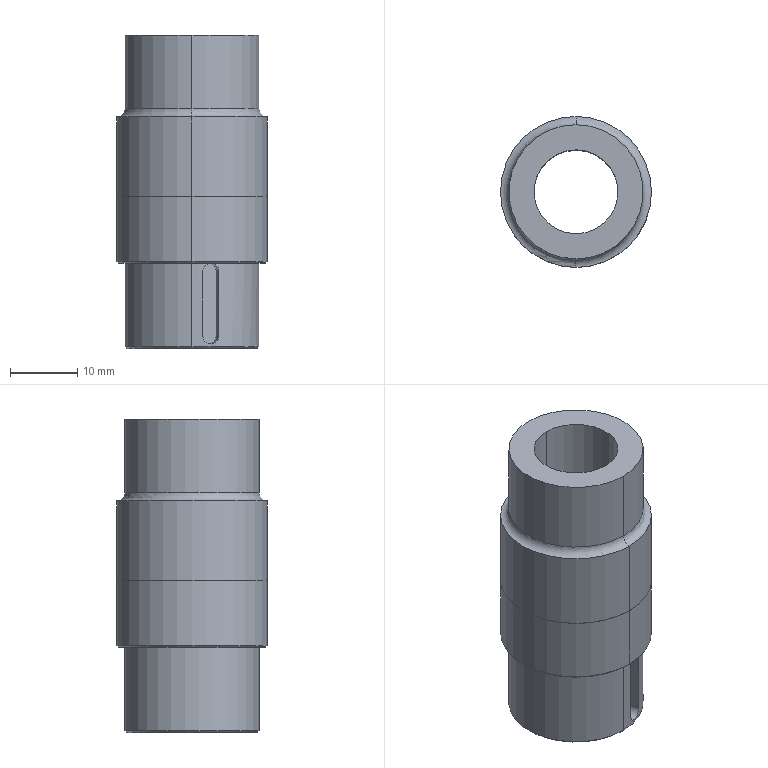Part | STEP file | 2026.6.15-Main Assembly图.sldasm-Part-96 | 1 solid | 32 faces | box 22.5 x 22.5 x 46.645 mm | volume 10487 mm3 | cylinder 16 | plane 8 | cone 6 | torus 2 | commonest cylinder face diameters 2.5 x4 20 x4 12.5 x2 14 x2 22.45 x2 22.5 x2
STEP:
#1=CARTESIAN_POINT('',(-1569.631,1414.394,3480.447));
#2=VERTEX_POINT('',#1);
#3=CARTESIAN_POINT('',(-1569.631,1414.394,3480.441));
#4=VERTEX_POINT('',#3);
#5=CARTESIAN_POINT('',(-1569.631,1414.394,3480.447));
#6=CARTESIAN_POINT('',(-1569.631,1414.394,3480.445));
#7=CARTESIAN_POINT('',(-1569.631,1414.394,3480.443));
#8=CARTESIAN_POINT('',(-1569.631,1414.394,3480.441));
#9=B_SPLINE_CURVE_WITH_KNOTS('',3,(#5,#6,#7,#8),.UNSPECIFIED.,.F.,.F.,(4,4),(0.,0.000005656),.UNSPECIFIED.);
#10=EDGE_CURVE('',#2,#4,#9,.T.);
#11=ORIENTED_EDGE('',*,*,#10,.T.);
#12=CARTESIAN_POINT('',(-1570.033,1415.758,3480.441));
#13=VERTEX_POINT('',#12);
#14=CARTESIAN_POINT('',(-1570.033,1415.758,3480.441));
#15=DIRECTION('',(-0.2829,0.9592,0.));
#16=VECTOR('',#15,1000.);
#17=LINE('',#14,#16);
#18=EDGE_CURVE('',#4,#13,#17,.T.);
#19=ORIENTED_EDGE('',*,*,#18,.T.);
#20=CARTESIAN_POINT('',(-1570.033,1415.758,3480.447));
#21=VERTEX_POINT('',#20);
#22=CARTESIAN_POINT('',(-1568.834,1416.111,3480.447));
#23=DIRECTION('',(0.2829,-0.9592,0.));
#24=DIRECTION('',(-0.9591,-0.2829,-0.004589));
#25=AXIS2_PLACEMENT_3D('',#22,#23,#24);
#26=CIRCLE('',#25,1.25);
#27=EDGE_CURVE('',#21,#13,#26,.T.);
#28=ORIENTED_EDGE('',*,*,#27,.F.);
#29=CARTESIAN_POINT('',(-1570.033,1415.758,3480.447));
#30=DIRECTION('',(-0.2829,0.9592,0.));
#31=VECTOR('',#30,1000.);
#32=LINE('',#29,#31);
#33=EDGE_CURVE('',#2,#21,#32,.T.);
#34=ORIENTED_EDGE('',*,*,#33,.F.);
#35=EDGE_LOOP('',(#11,#19,#28,#34));
#36=FACE_OUTER_BOUND('',#35,.T.);
#37=CARTESIAN_POINT('',(-1568.834,1416.111,3480.447));
#38=DIRECTION('',(-0.2829,0.9592,0.));
#39=DIRECTION('',(-0.9591,-0.2829,-0.004589));
#40=AXIS2_PLACEMENT_3D('',#37,#38,#39);
#41=CYLINDRICAL_SURFACE('',#40,1.25);
#42=ADVANCED_FACE('',(#36),#41,.F.);
#43=CARTESIAN_POINT('',(-1567.635,1416.465,3489.953));
#44=VERTEX_POINT('',#43);
#45=CARTESIAN_POINT('',(-1570.033,1415.758,3489.947));
#46=VERTEX_POINT('',#45);
#47=CARTESIAN_POINT('',(-1568.834,1416.111,3489.947));
#48=DIRECTION('',(0.2829,-0.9592,0.));
#49=DIRECTION('',(-0.9591,-0.2829,-0.004589));
#50=AXIS2_PLACEMENT_3D('',#47,#48,#49);
#51=CIRCLE('',#50,1.25);
#52=EDGE_CURVE('',#44,#46,#51,.T.);
#53=ORIENTED_EDGE('',*,*,#52,.F.);
#54=CARTESIAN_POINT('',(-1567.233,1415.102,3489.953));
#55=VERTEX_POINT('',#54);
#56=CARTESIAN_POINT('',(-1567.635,1416.465,3489.953));
#57=DIRECTION('',(0.2829,-0.9592,0.));
#58=VECTOR('',#57,1000.);
#59=LINE('',#56,#58);
#60=EDGE_CURVE('',#44,#55,#59,.T.);
#61=ORIENTED_EDGE('',*,*,#60,.T.);
#62=CARTESIAN_POINT('',(-1568.41,1414.673,3491.197));
#63=VERTEX_POINT('',#62);
#64=CARTESIAN_POINT('',(-1567.233,1415.102,3489.953));
#65=CARTESIAN_POINT('',(-1567.234,1415.101,3490.117));
#66=CARTESIAN_POINT('',(-1567.264,1415.088,3490.279));
#67=CARTESIAN_POINT('',(-1567.381,1415.038,3490.58));
#68=CARTESIAN_POINT('',(-1567.467,1415.002,3490.718));
#69=CARTESIAN_POINT('',(-1567.683,1414.917,3490.948));
#70=CARTESIAN_POINT('',(-1567.813,1414.868,3491.04));
#71=CARTESIAN_POINT('',(-1568.097,1414.769,3491.164));
#72=CARTESIAN_POINT('',(-1568.253,1414.719,3491.197));
#73=CARTESIAN_POINT('',(-1568.41,1414.673,3491.197));
#74=B_SPLINE_CURVE_WITH_KNOTS('',3,(#64,#65,#66,#67,#68,#69,#70,#71,#72,#73),.UNSPECIFIED.,.F.,.F.,(4,2,2,2,4),(0.000005656,0.0004933,0.000981,0.001469,0.001956),.UNSPECIFIED.);
#75=EDGE_CURVE('',#55,#63,#74,.T.);
#76=ORIENTED_EDGE('',*,*,#75,.T.);
#77=CARTESIAN_POINT('',(-1569.631,1414.394,3489.947));
#78=VERTEX_POINT('',#77);
#79=CARTESIAN_POINT('',(-1568.41,1414.673,3491.197));
#80=CARTESIAN_POINT('',(-1568.488,1414.65,3491.197));
#81=CARTESIAN_POINT('',(-1568.568,1414.627,3491.189));
#82=CARTESIAN_POINT('',(-1568.722,1414.586,3491.157));
#83=CARTESIAN_POINT('',(-1568.798,1414.566,3491.133));
#84=CARTESIAN_POINT('',(-1569.019,1414.513,3491.039));
#85=CARTESIAN_POINT('',(-1569.153,1414.483,3490.947));
#86=CARTESIAN_POINT('',(-1569.383,1414.437,3490.714));
#87=CARTESIAN_POINT('',(-1569.474,1414.421,3490.577));
#88=CARTESIAN_POINT('',(-1569.598,1414.4,3490.275));
#89=CARTESIAN_POINT('',(-1569.631,1414.394,3490.112));
#90=CARTESIAN_POINT('',(-1569.631,1414.394,3489.947));
#91=B_SPLINE_CURVE_WITH_KNOTS('',3,(#79,#80,#81,#82,#83,#84,#85,#86,#87,#88,#89,#90),.UNSPECIFIED.,.F.,.F.,(4,2,2,2,2,4),(0.001956,0.002201,0.002445,0.002934,0.003422,0.003911),.UNSPECIFIED.);
#92=EDGE_CURVE('',#63,#78,#91,.T.);
#93=ORIENTED_EDGE('',*,*,#92,.T.);
#94=CARTESIAN_POINT('',(-1570.033,1415.758,3489.947));
#95=DIRECTION('',(0.2829,-0.9592,0.));
#96=VECTOR('',#95,1000.);
#97=LINE('',#94,#96);
#98=EDGE_CURVE('',#46,#78,#97,.T.);
#99=ORIENTED_EDGE('',*,*,#98,.F.);
#100=EDGE_LOOP('',(#53,#61,#76,#93,#99));
#101=FACE_OUTER_BOUND('',#100,.T.);
#102=CARTESIAN_POINT('',(-1568.834,1416.111,3489.947));
#103=DIRECTION('',(0.2829,-0.9592,0.));
#104=DIRECTION('',(0.9591,0.2829,0.004589));
#105=AXIS2_PLACEMENT_3D('',#102,#103,#104);
#106=CYLINDRICAL_SURFACE('',#105,1.25);
#107=ADVANCED_FACE('',(#101),#106,.F.);
#108=CARTESIAN_POINT('',(-1571.247,1413.014,3501.197));
#109=VERTEX_POINT('',#108);
#110=CARTESIAN_POINT('',(-1571.23,1435.514,3501.197));
#111=VERTEX_POINT('',#110);
#112=CARTESIAN_POINT('',(-1571.238,1424.264,3501.197));
#113=DIRECTION('',(0.,0.,1.));
#114=DIRECTION('',(-0.0007664,-1.,0.));
#115=AXIS2_PLACEMENT_3D('',#112,#113,#114);
#116=CIRCLE('',#115,11.25);
#117=EDGE_CURVE('',#109,#111,#116,.T.);
#118=ORIENTED_EDGE('',*,*,#117,.T.);
#119=CARTESIAN_POINT('',(-1571.23,1435.514,3512.997));
#120=VERTEX_POINT('',#119);
#121=CARTESIAN_POINT('',(-1571.23,1435.514,3478.747));
#122=DIRECTION('',(0.,0.,1.));
#123=VECTOR('',#122,1000.);
#124=LINE('',#121,#123);
#125=EDGE_CURVE('',#111,#120,#124,.T.);
#126=ORIENTED_EDGE('',*,*,#125,.T.);
#127=CARTESIAN_POINT('',(-1571.247,1413.014,3512.997));
#128=VERTEX_POINT('',#127);
#129=CARTESIAN_POINT('',(-1571.238,1424.264,3512.997));
#130=DIRECTION('',(0.,0.,1.));
#131=DIRECTION('',(-0.0007664,-1.,0.));
#132=AXIS2_PLACEMENT_3D('',#129,#130,#131);
#133=CIRCLE('',#132,11.25);
#134=EDGE_CURVE('',#128,#120,#133,.T.);
#135=ORIENTED_EDGE('',*,*,#134,.F.);
#136=CARTESIAN_POINT('',(-1571.247,1413.014,3478.747));
#137=DIRECTION('',(0.,0.,1.));
#138=VECTOR('',#137,1000.);
#139=LINE('',#136,#138);
#140=EDGE_CURVE('',#109,#128,#139,.T.);
#141=ORIENTED_EDGE('',*,*,#140,.F.);
#142=EDGE_LOOP('',(#118,#126,#135,#141));
#143=FACE_OUTER_BOUND('',#142,.T.);
#144=CARTESIAN_POINT('',(-1571.238,1424.264,3478.747));
#145=DIRECTION('',(0.,0.,1.));
#146=DIRECTION('',(-0.0007664,-1.,0.));
#147=AXIS2_PLACEMENT_3D('',#144,#145,#146);
#148=CYLINDRICAL_SURFACE('',#147,11.25);
#149=ADVANCED_FACE('',(#143),#148,.T.);
#150=CARTESIAN_POINT('',(-1571.231,1434.264,3514.247));
#151=VERTEX_POINT('',#150);
#152=CARTESIAN_POINT('',(-1571.246,1414.264,3514.247));
#153=VERTEX_POINT('',#152);
#154=CARTESIAN_POINT('',(-1571.238,1424.264,3514.247));
#155=DIRECTION('',(0.,0.,1.));
#156=DIRECTION('',(-0.0007664,-1.,0.));
#157=AXIS2_PLACEMENT_3D('',#154,#155,#156);
#158=CIRCLE('',#157,10.);
#159=EDGE_CURVE('',#151,#153,#158,.T.);
#160=ORIENTED_EDGE('',*,*,#159,.F.);
#161=CARTESIAN_POINT('',(-1571.23,1435.514,3514.247));
#162=DIRECTION('',(1.,-0.0007664,0.));
#163=DIRECTION('',(0.0007664,1.,0.));
#164=AXIS2_PLACEMENT_3D('',#161,#162,#163);
#165=CIRCLE('',#164,1.25);
#166=EDGE_CURVE('',#151,#120,#165,.T.);
#167=ORIENTED_EDGE('',*,*,#166,.T.);
#168=CARTESIAN_POINT('',(-1571.238,1424.264,3512.997));
#169=DIRECTION('',(0.,0.,1.));
#170=DIRECTION('',(-0.0007664,-1.,0.));
#171=AXIS2_PLACEMENT_3D('',#168,#169,#170);
#172=CIRCLE('',#171,11.25);
#173=EDGE_CURVE('',#120,#128,#172,.T.);
#174=ORIENTED_EDGE('',*,*,#173,.T.);
#175=CARTESIAN_POINT('',(-1571.247,1413.014,3514.247));
#176=DIRECTION('',(-1.,0.0007664,0.));
#177=DIRECTION('',(-0.0007664,-1.,0.));
#178=AXIS2_PLACEMENT_3D('',#175,#176,#177);
#179=CIRCLE('',#178,1.25);
#180=EDGE_CURVE('',#153,#128,#179,.T.);
#181=ORIENTED_EDGE('',*,*,#180,.F.);
#182=EDGE_LOOP('',(#160,#167,#174,#181));
#183=FACE_OUTER_BOUND('',#182,.T.);
#184=CARTESIAN_POINT('',(-1571.238,1424.264,3514.247));
#185=DIRECTION('',(0.,0.,1.));
#186=DIRECTION('',(-0.0007664,-1.,0.));
#187=AXIS2_PLACEMENT_3D('',#184,#185,#186);
#188=TOROIDAL_SURFACE('',#187,11.25,1.25);
#189=ADVANCED_FACE('',(#183),#188,.F.);
#190=CARTESIAN_POINT('',(-1571.238,1424.264,3514.247));
#191=DIRECTION('',(0.,0.,1.));
#192=DIRECTION('',(-0.0007664,-1.,0.));
#193=AXIS2_PLACEMENT_3D('',#190,#191,#192);
#194=CIRCLE('',#193,10.);
#195=EDGE_CURVE('',#153,#151,#194,.T.);
#196=ORIENTED_EDGE('',*,*,#195,.T.);
#197=CARTESIAN_POINT('',(-1571.231,1434.264,3525.142));
#198=VERTEX_POINT('',#197);
#199=CARTESIAN_POINT('',(-1571.231,1434.264,3478.747));
#200=DIRECTION('',(0.,0.,1.));
#201=VECTOR('',#200,1000.);
#202=LINE('',#199,#201);
#203=EDGE_CURVE('',#151,#198,#202,.T.);
#204=ORIENTED_EDGE('',*,*,#203,.T.);
#205=CARTESIAN_POINT('',(-1571.246,1414.264,3525.142));
#206=VERTEX_POINT('',#205);
#207=CARTESIAN_POINT('',(-1571.238,1424.264,3525.142));
#208=DIRECTION('',(0.,0.,-1.));
#209=DIRECTION('',(-1.,0.,0.));
#210=AXIS2_PLACEMENT_3D('',#207,#208,#209);
#211=CIRCLE('',#210,10.);
#212=EDGE_CURVE('',#198,#206,#211,.T.);
#213=ORIENTED_EDGE('',*,*,#212,.T.);
#214=CARTESIAN_POINT('',(-1571.246,1414.264,3478.747));
#215=DIRECTION('',(0.,0.,1.));
#216=VECTOR('',#215,1000.);
#217=LINE('',#214,#216);
#218=EDGE_CURVE('',#153,#206,#217,.T.);
#219=ORIENTED_EDGE('',*,*,#218,.F.);
#220=EDGE_LOOP('',(#196,#204,#213,#219));
#221=FACE_OUTER_BOUND('',#220,.T.);
#222=CARTESIAN_POINT('',(-1571.238,1424.264,3478.747));
#223=DIRECTION('',(0.,0.,1.));
#224=DIRECTION('',(-0.0007664,-1.,0.));
#225=AXIS2_PLACEMENT_3D('',#222,#223,#224);
#226=CYLINDRICAL_SURFACE('',#225,10.);
#227=ADVANCED_FACE('',(#221),#226,.T.);
#228=CARTESIAN_POINT('',(-1571.233,1430.514,3485.497));
#229=VERTEX_POINT('',#228);
#230=CARTESIAN_POINT('',(-1571.243,1418.014,3485.497));
#231=VERTEX_POINT('',#230);
#232=CARTESIAN_POINT('',(-1571.238,1424.264,3485.497));
#233=DIRECTION('',(0.,0.,1.));
#234=DIRECTION('',(-0.0007664,-1.,0.));
#235=AXIS2_PLACEMENT_3D('',#232,#233,#234);
#236=CIRCLE('',#235,6.25);
#237=EDGE_CURVE('',#229,#231,#236,.T.);
#238=ORIENTED_EDGE('',*,*,#237,.F.);
#239=CARTESIAN_POINT('',(-1571.233,1430.514,3525.142));
#240=VERTEX_POINT('',#239);
#241=CARTESIAN_POINT('',(-1571.233,1430.514,3478.747));
#242=DIRECTION('',(0.,0.,1.));
#243=VECTOR('',#242,1000.);
#244=LINE('',#241,#243);
#245=EDGE_CURVE('',#229,#240,#244,.T.);
#246=ORIENTED_EDGE('',*,*,#245,.T.);
#247=CARTESIAN_POINT('',(-1571.243,1418.014,3525.142));
#248=VERTEX_POINT('',#247);
#249=CARTESIAN_POINT('',(-1571.238,1424.264,3525.142));
#250=DIRECTION('',(0.,0.,1.));
#251=DIRECTION('',(-1.,0.,0.));
#252=AXIS2_PLACEMENT_3D('',#249,#250,#251);
#253=CIRCLE('',#252,6.25);
#254=EDGE_CURVE('',#240,#248,#253,.T.);
#255=ORIENTED_EDGE('',*,*,#254,.T.);
#256=CARTESIAN_POINT('',(-1571.243,1418.014,3478.747));
#257=DIRECTION('',(0.,0.,1.));
#258=VECTOR('',#257,1000.);
#259=LINE('',#256,#258);
#260=EDGE_CURVE('',#231,#248,#259,.T.);
#261=ORIENTED_EDGE('',*,*,#260,.F.);
#262=EDGE_LOOP('',(#238,#246,#255,#261));
#263=FACE_OUTER_BOUND('',#262,.T.);
#264=CARTESIAN_POINT('',(-1571.238,1424.264,3478.747));
#265=DIRECTION('',(0.,0.,1.));
#266=DIRECTION('',(-0.0007664,-1.,0.));
#267=AXIS2_PLACEMENT_3D('',#264,#265,#266);
#268=CYLINDRICAL_SURFACE('',#267,6.25);
#269=ADVANCED_FACE('',(#263),#268,.F.);
#270=CARTESIAN_POINT('',(-1571.233,1431.264,3478.747));
#271=VERTEX_POINT('',#270);
#272=CARTESIAN_POINT('',(-1571.244,1417.264,3478.747));
#273=VERTEX_POINT('',#272);
#274=CARTESIAN_POINT('',(-1571.238,1424.264,3478.747));
#275=DIRECTION('',(0.,0.,1.));
#276=DIRECTION('',(-0.0007664,-1.,0.));
#277=AXIS2_PLACEMENT_3D('',#274,#275,#276);
#278=CIRCLE('',#277,7.);
#279=EDGE_CURVE('',#271,#273,#278,.T.);
#280=ORIENTED_EDGE('',*,*,#279,.F.);
#281=CARTESIAN_POINT('',(-1571.233,1431.264,3485.497));
#282=VERTEX_POINT('',#281);
#283=CARTESIAN_POINT('',(-1571.233,1431.264,3478.747));
#284=DIRECTION('',(0.,0.,1.));
#285=VECTOR('',#284,1000.);
#286=LINE('',#283,#285);
#287=EDGE_CURVE('',#271,#282,#286,.T.);
#288=ORIENTED_EDGE('',*,*,#287,.T.);
#289=CARTESIAN_POINT('',(-1571.244,1417.264,3485.497));
#290=VERTEX_POINT('',#289);
#291=CARTESIAN_POINT('',(-1571.238,1424.264,3485.497));
#292=DIRECTION('',(0.,0.,1.));
#293=DIRECTION('',(-0.0007664,-1.,0.));
#294=AXIS2_PLACEMENT_3D('',#291,#292,#293);
#295=CIRCLE('',#294,7.);
#296=EDGE_CURVE('',#282,#290,#295,.T.);
#297=ORIENTED_EDGE('',*,*,#296,.T.);
#298=CARTESIAN_POINT('',(-1571.244,1417.264,3478.747));
#299=DIRECTION('',(0.,0.,1.));
#300=VECTOR('',#299,1000.);
#301=LINE('',#298,#300);
#302=EDGE_CURVE('',#273,#290,#301,.T.);
#303=ORIENTED_EDGE('',*,*,#302,.F.);
#304=EDGE_LOOP('',(#280,#288,#297,#303));
#305=FACE_OUTER_BOUND('',#304,.T.);
#306=CARTESIAN_POINT('',(-1571.238,1424.264,3478.747));
#307=DIRECTION('',(0.,0.,1.));
#308=DIRECTION('',(-0.0007664,-1.,0.));
#309=AXIS2_PLACEMENT_3D('',#306,#307,#308);
#310=CYLINDRICAL_SURFACE('',#309,7.);
#311=ADVANCED_FACE('',(#305),#310,.F.);
#312=ORIENTED_EDGE('',*,*,#279,.T.);
#313=CARTESIAN_POINT('',(-1571.244,1417.014,3478.497));
#314=VERTEX_POINT('',#313);
#315=CARTESIAN_POINT('',(-1571.244,1417.014,3478.497));
#316=DIRECTION('',(-0.000542,-0.7071,-0.7071));
#317=VECTOR('',#316,1000.);
#318=LINE('',#315,#317);
#319=EDGE_CURVE('',#273,#314,#318,.T.);
#320=ORIENTED_EDGE('',*,*,#319,.T.);
#321=CARTESIAN_POINT('',(-1571.233,1431.514,3478.497));
#322=VERTEX_POINT('',#321);
#323=CARTESIAN_POINT('',(-1571.238,1424.264,3478.497));
#324=DIRECTION('',(0.,0.,1.));
#325=DIRECTION('',(-0.0007664,-1.,0.));
#326=AXIS2_PLACEMENT_3D('',#323,#324,#325);
#327=CIRCLE('',#326,7.25);
#328=EDGE_CURVE('',#322,#314,#327,.T.);
#329=ORIENTED_EDGE('',*,*,#328,.F.);
#330=CARTESIAN_POINT('',(-1571.233,1431.514,3478.497));
#331=DIRECTION('',(0.000542,0.7071,-0.7071));
#332=VECTOR('',#331,1000.);
#333=LINE('',#330,#332);
#334=EDGE_CURVE('',#271,#322,#333,.T.);
#335=ORIENTED_EDGE('',*,*,#334,.F.);
#336=EDGE_LOOP('',(#312,#320,#329,#335));
#337=FACE_OUTER_BOUND('',#336,.T.);
#338=CARTESIAN_POINT('',(-1571.238,1424.264,3478.497));
#339=DIRECTION('',(0.,0.,-1.));
#340=DIRECTION('',(0.0007664,1.,0.));
#341=AXIS2_PLACEMENT_3D('',#338,#339,#340);
#342=CONICAL_SURFACE('',#341,7.25,0.7854);
#343=ADVANCED_FACE('',(#337),#342,.F.);
#344=CARTESIAN_POINT('',(-1571.246,1414.514,3478.497));
#345=VERTEX_POINT('',#344);
#346=CARTESIAN_POINT('',(-1571.231,1434.014,3478.497));
#347=VERTEX_POINT('',#346);
#348=CARTESIAN_POINT('',(-1571.238,1424.264,3478.497));
#349=DIRECTION('',(0.,0.,1.));
#350=DIRECTION('',(-0.0007664,-1.,0.));
#351=AXIS2_PLACEMENT_3D('',#348,#349,#350);
#352=CIRCLE('',#351,9.75);
#353=EDGE_CURVE('',#345,#347,#352,.T.);
#354=ORIENTED_EDGE('',*,*,#353,.T.);
#355=CARTESIAN_POINT('',(-1571.231,1434.264,3478.747));
#356=VERTEX_POINT('',#355);
#357=CARTESIAN_POINT('',(-1571.231,1434.264,3478.747));
#358=DIRECTION('',(0.000542,0.7071,0.7071));
#359=VECTOR('',#358,1000.);
#360=LINE('',#357,#359);
#361=EDGE_CURVE('',#347,#356,#360,.T.);
#362=ORIENTED_EDGE('',*,*,#361,.T.);
#363=CARTESIAN_POINT('',(-1571.246,1414.264,3478.747));
#364=VERTEX_POINT('',#363);
#365=CARTESIAN_POINT('',(-1571.238,1424.264,3478.747));
#366=DIRECTION('',(0.,0.,1.));
#367=DIRECTION('',(-0.0007664,-1.,0.));
#368=AXIS2_PLACEMENT_3D('',#365,#366,#367);
#369=CIRCLE('',#368,10.);
#370=EDGE_CURVE('',#364,#356,#369,.T.);
#371=ORIENTED_EDGE('',*,*,#370,.F.);
#372=CARTESIAN_POINT('',(-1571.246,1414.264,3478.747));
#373=DIRECTION('',(-0.000542,-0.7071,0.7071));
#374=VECTOR('',#373,1000.);
#375=LINE('',#372,#374);
#376=EDGE_CURVE('',#345,#364,#375,.T.);
#377=ORIENTED_EDGE('',*,*,#376,.F.);
#378=EDGE_LOOP('',(#354,#362,#371,#377));
#379=FACE_OUTER_BOUND('',#378,.T.);
#380=CARTESIAN_POINT('',(-1571.238,1424.264,3478.747));
#381=DIRECTION('',(0.,0.,1.));
#382=DIRECTION('',(-0.0007664,-1.,0.));
#383=AXIS2_PLACEMENT_3D('',#380,#381,#382);
#384=CONICAL_SURFACE('',#383,10.,0.7854);
#385=ADVANCED_FACE('',(#379),#384,.T.);
#386=ORIENTED_EDGE('',*,*,#370,.T.);
#387=CARTESIAN_POINT('',(-1571.231,1434.264,3491.197));
#388=VERTEX_POINT('',#387);
#389=CARTESIAN_POINT('',(-1571.231,1434.264,3478.747));
#390=DIRECTION('',(0.,0.,1.));
#391=VECTOR('',#390,1000.);
#392=LINE('',#389,#391);
#393=EDGE_CURVE('',#356,#388,#392,.T.);
#394=ORIENTED_EDGE('',*,*,#393,.T.);
#395=CARTESIAN_POINT('',(-1571.238,1424.264,3491.197));
#396=DIRECTION('',(0.,0.,1.));
#397=DIRECTION('',(-0.0007664,-1.,0.));
#398=AXIS2_PLACEMENT_3D('',#395,#396,#397);
#399=CIRCLE('',#398,10.);
#400=EDGE_CURVE('',#63,#388,#399,.T.);
#401=ORIENTED_EDGE('',*,*,#400,.F.);
#402=ORIENTED_EDGE('',*,*,#75,.F.);
#403=CARTESIAN_POINT('',(-1567.233,1415.102,3489.947));
#404=VERTEX_POINT('',#403);
#405=CARTESIAN_POINT('',(-1567.233,1415.102,3489.947));
#406=CARTESIAN_POINT('',(-1567.233,1415.102,3489.949));
#407=CARTESIAN_POINT('',(-1567.233,1415.102,3489.951));
#408=CARTESIAN_POINT('',(-1567.233,1415.102,3489.953));
#409=B_SPLINE_CURVE_WITH_KNOTS('',3,(#405,#406,#407,#408),.UNSPECIFIED.,.F.,.F.,(4,4),(0.,0.000005656),.UNSPECIFIED.);
#410=EDGE_CURVE('',#404,#55,#409,.T.);
#411=ORIENTED_EDGE('',*,*,#410,.F.);
#412=CARTESIAN_POINT('',(-1567.233,1415.102,3480.447));
#413=VERTEX_POINT('',#412);
#414=CARTESIAN_POINT('',(-1567.233,1415.102,3478.747));
#415=DIRECTION('',(0.,0.,-1.));
#416=VECTOR('',#415,1000.);
#417=LINE('',#414,#416);
#418=EDGE_CURVE('',#404,#413,#417,.T.);
#419=ORIENTED_EDGE('',*,*,#418,.T.);
#420=CARTESIAN_POINT('',(-1569.631,1414.394,3480.441));
#421=CARTESIAN_POINT('',(-1569.63,1414.394,3480.276));
#422=CARTESIAN_POINT('',(-1569.597,1414.4,3480.114));
#423=CARTESIAN_POINT('',(-1569.471,1414.421,3479.813));
#424=CARTESIAN_POINT('',(-1569.379,1414.438,3479.675));
#425=CARTESIAN_POINT('',(-1569.152,1414.484,3479.445));
#426=CARTESIAN_POINT('',(-1569.015,1414.513,3479.353));
#427=CARTESIAN_POINT('',(-1568.723,1414.585,3479.229));
#428=CARTESIAN_POINT('',(-1568.564,1414.627,3479.197));
#429=CARTESIAN_POINT('',(-1568.33,1414.696,3479.197));
#430=CARTESIAN_POINT('',(-1568.251,1414.721,3479.205));
#431=CARTESIAN_POINT('',(-1568.098,1414.77,3479.237));
#432=CARTESIAN_POINT('',(-1568.024,1414.795,3479.261));
#433=CARTESIAN_POINT('',(-1567.81,1414.869,3479.355));
#434=CARTESIAN_POINT('',(-1567.681,1414.918,3479.447));
#435=CARTESIAN_POINT('',(-1567.464,1415.003,3479.68));
#436=CARTESIAN_POINT('',(-1567.379,1415.039,3479.817));
#437=CARTESIAN_POINT('',(-1567.263,1415.088,3480.119));
#438=CARTESIAN_POINT('',(-1567.233,1415.102,3480.282));
#439=CARTESIAN_POINT('',(-1567.233,1415.102,3480.447));
#440=B_SPLINE_CURVE_WITH_KNOTS('',3,(#420,#421,#422,#423,#424,#425,#426,#427,#428,#429,#430,#431,#432,#433,#434,#435,#436,#437,#438,#439),.UNSPECIFIED.,.F.,.F.,(4,2,2,2,2,2,2,2,2,4),(0.000005656,0.0004938,0.000982,0.00147,0.001958,0.002202,0.002446,0.002935,0.003423,0.003911),.UNSPECIFIED.);
#441=EDGE_CURVE('',#4,#413,#440,.T.);
#442=ORIENTED_EDGE('',*,*,#441,.F.);
#443=ORIENTED_EDGE('',*,*,#10,.F.);
#444=CARTESIAN_POINT('',(-1569.631,1414.394,3478.747));
#445=DIRECTION('',(0.,0.,1.));
#446=VECTOR('',#445,1000.);
#447=LINE('',#444,#446);
#448=EDGE_CURVE('',#2,#78,#447,.T.);
#449=ORIENTED_EDGE('',*,*,#448,.T.);
#450=ORIENTED_EDGE('',*,*,#92,.F.);
#451=CARTESIAN_POINT('',(-1571.246,1414.264,3491.197));
#452=VERTEX_POINT('',#451);
#453=CARTESIAN_POINT('',(-1571.238,1424.264,3491.197));
#454=DIRECTION('',(0.,0.,1.));
#455=DIRECTION('',(-0.0007664,-1.,0.));
#456=AXIS2_PLACEMENT_3D('',#453,#454,#455);
#457=CIRCLE('',#456,10.);
#458=EDGE_CURVE('',#452,#63,#457,.T.);
#459=ORIENTED_EDGE('',*,*,#458,.F.);
#460=CARTESIAN_POINT('',(-1571.246,1414.264,3478.747));
#461=DIRECTION('',(0.,0.,1.));
#462=VECTOR('',#461,1000.);
#463=LINE('',#460,#462);
#464=EDGE_CURVE('',#364,#452,#463,.T.);
#465=ORIENTED_EDGE('',*,*,#464,.F.);
#466=EDGE_LOOP('',(#386,#394,#401,#402,#411,#419,#442,#443,#449,#450,#459,#465));
#467=FACE_OUTER_BOUND('',#466,.T.);
#468=CARTESIAN_POINT('',(-1571.238,1424.264,3478.747));
#469=DIRECTION('',(0.,0.,1.));
#470=DIRECTION('',(-0.0007664,-1.,0.));
#471=AXIS2_PLACEMENT_3D('',#468,#469,#470);
#472=CYLINDRICAL_SURFACE('',#471,10.);
#473=ADVANCED_FACE('',(#467),#472,.T.);
#474=CARTESIAN_POINT('',(-1571.247,1413.289,3491.197));
#475=VERTEX_POINT('',#474);
#476=CARTESIAN_POINT('',(-1571.23,1435.239,3491.197));
#477=VERTEX_POINT('',#476);
#478=CARTESIAN_POINT('',(-1571.238,1424.264,3491.197));
#479=DIRECTION('',(0.,0.,1.));
#480=DIRECTION('',(-0.0007664,-1.,0.));
#481=AXIS2_PLACEMENT_3D('',#478,#479,#480);
#482=CIRCLE('',#481,10.975);
#483=EDGE_CURVE('',#475,#477,#482,.T.);
#484=ORIENTED_EDGE('',*,*,#483,.T.);
#485=CARTESIAN_POINT('',(-1571.23,1435.489,3491.447));
#486=VERTEX_POINT('',#485);
#487=CARTESIAN_POINT('',(-1571.23,1435.489,3491.447));
#488=DIRECTION('',(0.000542,0.7071,0.7071));
#489=VECTOR('',#488,1000.);
#490=LINE('',#487,#489);
#491=EDGE_CURVE('',#477,#486,#490,.T.);
#492=ORIENTED_EDGE('',*,*,#491,.T.);
#493=CARTESIAN_POINT('',(-1571.247,1413.039,3491.447));
#494=VERTEX_POINT('',#493);
#495=CARTESIAN_POINT('',(-1571.238,1424.264,3491.447));
#496=DIRECTION('',(0.,0.,1.));
#497=DIRECTION('',(-0.0007664,-1.,0.));
#498=AXIS2_PLACEMENT_3D('',#495,#496,#497);
#499=CIRCLE('',#498,11.225);
#500=EDGE_CURVE('',#494,#486,#499,.T.);
#501=ORIENTED_EDGE('',*,*,#500,.F.);
#502=CARTESIAN_POINT('',(-1571.247,1413.039,3491.447));
#503=DIRECTION('',(-0.000542,-0.7071,0.7071));
#504=VECTOR('',#503,1000.);
#505=LINE('',#502,#504);
#506=EDGE_CURVE('',#475,#494,#505,.T.);
#507=ORIENTED_EDGE('',*,*,#506,.F.);
#508=EDGE_LOOP('',(#484,#492,#501,#507));
#509=FACE_OUTER_BOUND('',#508,.T.);
#510=CARTESIAN_POINT('',(-1571.238,1424.264,3491.447));
#511=DIRECTION('',(0.,0.,1.));
#512=DIRECTION('',(-0.0007664,-1.,0.));
#513=AXIS2_PLACEMENT_3D('',#510,#511,#512);
#514=CONICAL_SURFACE('',#513,11.225,0.7854);
#515=ADVANCED_FACE('',(#509),#514,.T.);
#516=ORIENTED_EDGE('',*,*,#500,.T.);
#517=CARTESIAN_POINT('',(-1571.23,1435.489,3501.197));
#518=VERTEX_POINT('',#517);
#519=CARTESIAN_POINT('',(-1571.23,1435.489,3478.747));
#520=DIRECTION('',(0.,0.,1.));
#521=VECTOR('',#520,1000.);
#522=LINE('',#519,#521);
#523=EDGE_CURVE('',#486,#518,#522,.T.);
#524=ORIENTED_EDGE('',*,*,#523,.T.);
#525=CARTESIAN_POINT('',(-1571.247,1413.039,3501.197));
#526=VERTEX_POINT('',#525);
#527=CARTESIAN_POINT('',(-1571.238,1424.264,3501.197));
#528=DIRECTION('',(0.,0.,1.));
#529=DIRECTION('',(-0.0007664,-1.,0.));
#530=AXIS2_PLACEMENT_3D('',#527,#528,#529);
#531=CIRCLE('',#530,11.225);
#532=EDGE_CURVE('',#526,#518,#531,.T.);
#533=ORIENTED_EDGE('',*,*,#532,.F.);
#534=CARTESIAN_POINT('',(-1571.247,1413.039,3478.747));
#535=DIRECTION('',(0.,0.,1.));
#536=VECTOR('',#535,1000.);
#537=LINE('',#534,#536);
#538=EDGE_CURVE('',#494,#526,#537,.T.);
#539=ORIENTED_EDGE('',*,*,#538,.F.);
#540=EDGE_LOOP('',(#516,#524,#533,#539));
#541=FACE_OUTER_BOUND('',#540,.T.);
#542=CARTESIAN_POINT('',(-1571.238,1424.264,3478.747));
#543=DIRECTION('',(0.,0.,1.));
#544=DIRECTION('',(-0.0007664,-1.,0.));
#545=AXIS2_PLACEMENT_3D('',#542,#543,#544);
#546=CYLINDRICAL_SURFACE('',#545,11.225);
#547=ADVANCED_FACE('',(#541),#546,.T.);
#548=ORIENTED_EDGE('',*,*,#523,.F.);
#549=CARTESIAN_POINT('',(-1571.238,1424.264,3491.447));
#550=DIRECTION('',(0.,0.,1.));
#551=DIRECTION('',(-0.0007664,-1.,0.));
#552=AXIS2_PLACEMENT_3D('',#549,#550,#551);
#553=CIRCLE('',#552,11.225);
#554=EDGE_CURVE('',#486,#494,#553,.T.);
#555=ORIENTED_EDGE('',*,*,#554,.T.);
#556=ORIENTED_EDGE('',*,*,#538,.T.);
#557=CARTESIAN_POINT('',(-1571.238,1424.264,3501.197));
#558=DIRECTION('',(0.,0.,1.));
#559=DIRECTION('',(-0.0007664,-1.,0.));
#560=AXIS2_PLACEMENT_3D('',#557,#558,#559);
#561=CIRCLE('',#560,11.225);
#562=EDGE_CURVE('',#518,#526,#561,.T.);
#563=ORIENTED_EDGE('',*,*,#562,.F.);
#564=EDGE_LOOP('',(#548,#555,#556,#563));
#565=FACE_OUTER_BOUND('',#564,.T.);
#566=CARTESIAN_POINT('',(-1571.238,1424.264,3478.747));
#567=DIRECTION('',(0.,0.,1.));
#568=DIRECTION('',(-0.0007664,-1.,0.));
#569=AXIS2_PLACEMENT_3D('',#566,#567,#568);
#570=CYLINDRICAL_SURFACE('',#569,11.225);
#571=ADVANCED_FACE('',(#565),#570,.T.);
#572=ORIENTED_EDGE('',*,*,#491,.F.);
#573=CARTESIAN_POINT('',(-1571.238,1424.264,3491.197));
#574=DIRECTION('',(0.,0.,1.));
#575=DIRECTION('',(-0.0007664,-1.,0.));
#576=AXIS2_PLACEMENT_3D('',#573,#574,#575);
#577=CIRCLE('',#576,10.975);
#578=EDGE_CURVE('',#477,#475,#577,.T.);
#579=ORIENTED_EDGE('',*,*,#578,.T.);
#580=ORIENTED_EDGE('',*,*,#506,.T.);
#581=ORIENTED_EDGE('',*,*,#554,.F.);
#582=EDGE_LOOP('',(#572,#579,#580,#581));
#583=FACE_OUTER_BOUND('',#582,.T.);
#584=CARTESIAN_POINT('',(-1571.238,1424.264,3491.447));
#585=DIRECTION('',(0.,0.,1.));
#586=DIRECTION('',(-0.0007664,-1.,0.));
#587=AXIS2_PLACEMENT_3D('',#584,#585,#586);
#588=CONICAL_SURFACE('',#587,11.225,0.7854);
#589=ADVANCED_FACE('',(#583),#588,.T.);
#590=ORIENTED_EDGE('',*,*,#400,.T.);
#591=CARTESIAN_POINT('',(-1571.238,1424.264,3491.197));
#592=DIRECTION('',(0.,0.,1.));
#593=DIRECTION('',(-0.0007664,-1.,0.));
#594=AXIS2_PLACEMENT_3D('',#591,#592,#593);
#595=CIRCLE('',#594,10.);
#596=EDGE_CURVE('',#388,#452,#595,.T.);
#597=ORIENTED_EDGE('',*,*,#596,.T.);
#598=ORIENTED_EDGE('',*,*,#458,.T.);
#599=EDGE_LOOP('',(#590,#597,#598));
#600=FACE_BOUND('',#599,.T.);
#601=ORIENTED_EDGE('',*,*,#483,.F.);
#602=ORIENTED_EDGE('',*,*,#578,.F.);
#603=EDGE_LOOP('',(#601,#602));
#604=FACE_OUTER_BOUND('',#603,.T.);
#605=CARTESIAN_POINT('',(-1581.765,1421.16,3491.197));
#606=DIRECTION('',(0.,0.,-1.));
#607=DIRECTION('',(0.0007664,1.,0.));
#608=AXIS2_PLACEMENT_3D('',#605,#606,#607);
#609=PLANE('',#608);
#610=ADVANCED_FACE('',(#600,#604),#609,.T.);
#611=ORIENTED_EDGE('',*,*,#393,.F.);
#612=CARTESIAN_POINT('',(-1571.238,1424.264,3478.747));
#613=DIRECTION('',(0.,0.,1.));
#614=DIRECTION('',(-0.0007664,-1.,0.));
#615=AXIS2_PLACEMENT_3D('',#612,#613,#614);
#616=CIRCLE('',#615,10.);
#617=EDGE_CURVE('',#356,#364,#616,.T.);
#618=ORIENTED_EDGE('',*,*,#617,.T.);
#619=ORIENTED_EDGE('',*,*,#464,.T.);
#620=ORIENTED_EDGE('',*,*,#596,.F.);
#621=EDGE_LOOP('',(#611,#618,#619,#620));
#622=FACE_OUTER_BOUND('',#621,.T.);
#623=CARTESIAN_POINT('',(-1571.238,1424.264,3478.747));
#624=DIRECTION('',(0.,0.,1.));
#625=DIRECTION('',(-0.0007664,-1.,0.));
#626=AXIS2_PLACEMENT_3D('',#623,#624,#625);
#627=CYLINDRICAL_SURFACE('',#626,10.);
#628=ADVANCED_FACE('',(#622),#627,.T.);
#629=ORIENTED_EDGE('',*,*,#361,.F.);
#630=CARTESIAN_POINT('',(-1571.238,1424.264,3478.497));
#631=DIRECTION('',(0.,0.,1.));
#632=DIRECTION('',(-0.0007664,-1.,0.));
#633=AXIS2_PLACEMENT_3D('',#630,#631,#632);
#634=CIRCLE('',#633,9.75);
#635=EDGE_CURVE('',#347,#345,#634,.T.);
#636=ORIENTED_EDGE('',*,*,#635,.T.);
#637=ORIENTED_EDGE('',*,*,#376,.T.);
#638=ORIENTED_EDGE('',*,*,#617,.F.);
#639=EDGE_LOOP('',(#629,#636,#637,#638));
#640=FACE_OUTER_BOUND('',#639,.T.);
#641=CARTESIAN_POINT('',(-1571.238,1424.264,3478.747));
#642=DIRECTION('',(0.,0.,1.));
#643=DIRECTION('',(-0.0007664,-1.,0.));
#644=AXIS2_PLACEMENT_3D('',#641,#642,#643);
#645=CONICAL_SURFACE('',#644,10.,0.7854);
#646=ADVANCED_FACE('',(#640),#645,.T.);
#647=ORIENTED_EDGE('',*,*,#328,.T.);
#648=CARTESIAN_POINT('',(-1571.238,1424.264,3478.497));
#649=DIRECTION('',(0.,0.,1.));
#650=DIRECTION('',(-0.0007664,-1.,0.));
#651=AXIS2_PLACEMENT_3D('',#648,#649,#650);
#652=CIRCLE('',#651,7.25);
#653=EDGE_CURVE('',#314,#322,#652,.T.);
#654=ORIENTED_EDGE('',*,*,#653,.T.);
#655=EDGE_LOOP('',(#647,#654));
#656=FACE_BOUND('',#655,.T.);
#657=ORIENTED_EDGE('',*,*,#353,.F.);
#658=ORIENTED_EDGE('',*,*,#635,.F.);
#659=EDGE_LOOP('',(#657,#658));
#660=FACE_OUTER_BOUND('',#659,.T.);
#661=CARTESIAN_POINT('',(-1580.59,1421.506,3478.497));
#662=DIRECTION('',(0.,0.,-1.));
#663=DIRECTION('',(0.0007664,1.,0.));
#664=AXIS2_PLACEMENT_3D('',#661,#662,#663);
#665=PLANE('',#664);
#666=ADVANCED_FACE('',(#656,#660),#665,.T.);
#667=ORIENTED_EDGE('',*,*,#319,.F.);
#668=CARTESIAN_POINT('',(-1571.238,1424.264,3478.747));
#669=DIRECTION('',(0.,0.,1.));
#670=DIRECTION('',(-0.0007664,-1.,0.));
#671=AXIS2_PLACEMENT_3D('',#668,#669,#670);
#672=CIRCLE('',#671,7.);
#673=EDGE_CURVE('',#273,#271,#672,.T.);
#674=ORIENTED_EDGE('',*,*,#673,.T.);
#675=ORIENTED_EDGE('',*,*,#334,.T.);
#676=ORIENTED_EDGE('',*,*,#653,.F.);
#677=EDGE_LOOP('',(#667,#674,#675,#676));
#678=FACE_OUTER_BOUND('',#677,.T.);
#679=CARTESIAN_POINT('',(-1571.238,1424.264,3478.497));
#680=DIRECTION('',(0.,0.,-1.));
#681=DIRECTION('',(0.0007664,1.,0.));
#682=AXIS2_PLACEMENT_3D('',#679,#680,#681);
#683=CONICAL_SURFACE('',#682,7.25,0.7854);
#684=ADVANCED_FACE('',(#678),#683,.F.);
#685=ORIENTED_EDGE('',*,*,#287,.F.);
#686=ORIENTED_EDGE('',*,*,#673,.F.);
#687=ORIENTED_EDGE('',*,*,#302,.T.);
#688=CARTESIAN_POINT('',(-1571.238,1424.264,3485.497));
#689=DIRECTION('',(0.,0.,1.));
#690=DIRECTION('',(-0.0007664,-1.,0.));
#691=AXIS2_PLACEMENT_3D('',#688,#689,#690);
#692=CIRCLE('',#691,7.);
#693=EDGE_CURVE('',#290,#282,#692,.T.);
#694=ORIENTED_EDGE('',*,*,#693,.T.);
#695=EDGE_LOOP('',(#685,#686,#687,#694));
#696=FACE_OUTER_BOUND('',#695,.T.);
#697=CARTESIAN_POINT('',(-1571.238,1424.264,3478.747));
#698=DIRECTION('',(0.,0.,1.));
#699=DIRECTION('',(-0.0007664,-1.,0.));
#700=AXIS2_PLACEMENT_3D('',#697,#698,#699);
#701=CYLINDRICAL_SURFACE('',#700,7.);
#702=ADVANCED_FACE('',(#696),#701,.F.);
#703=CARTESIAN_POINT('',(-1571.238,1424.264,3485.497));
#704=DIRECTION('',(0.,0.,1.));
#705=DIRECTION('',(-0.0007664,-1.,0.));
#706=AXIS2_PLACEMENT_3D('',#703,#704,#705);
#707=CIRCLE('',#706,6.25);
#708=EDGE_CURVE('',#231,#229,#707,.T.);
#709=ORIENTED_EDGE('',*,*,#708,.T.);
#710=ORIENTED_EDGE('',*,*,#237,.T.);
#711=EDGE_LOOP('',(#709,#710));
#712=FACE_BOUND('',#711,.T.);
#713=ORIENTED_EDGE('',*,*,#693,.F.);
#714=ORIENTED_EDGE('',*,*,#296,.F.);
#715=EDGE_LOOP('',(#713,#714));
#716=FACE_OUTER_BOUND('',#715,.T.);
#717=CARTESIAN_POINT('',(-1577.952,1422.284,3485.497));
#718=DIRECTION('',(0.,0.,-1.));
#719=DIRECTION('',(0.0007664,1.,0.));
#720=AXIS2_PLACEMENT_3D('',#717,#718,#719);
#721=PLANE('',#720);
#722=ADVANCED_FACE('',(#712,#716),#721,.T.);
#723=ORIENTED_EDGE('',*,*,#245,.F.);
#724=ORIENTED_EDGE('',*,*,#708,.F.);
#725=ORIENTED_EDGE('',*,*,#260,.T.);
#726=CARTESIAN_POINT('',(-1571.238,1424.264,3525.142));
#727=DIRECTION('',(0.,0.,1.));
#728=DIRECTION('',(-1.,0.,0.));
#729=AXIS2_PLACEMENT_3D('',#726,#727,#728);
#730=CIRCLE('',#729,6.25);
#731=EDGE_CURVE('',#248,#240,#730,.T.);
#732=ORIENTED_EDGE('',*,*,#731,.T.);
#733=EDGE_LOOP('',(#723,#724,#725,#732));
#734=FACE_OUTER_BOUND('',#733,.T.);
#735=CARTESIAN_POINT('',(-1571.238,1424.264,3478.747));
#736=DIRECTION('',(0.,0.,1.));
#737=DIRECTION('',(-0.0007664,-1.,0.));
#738=AXIS2_PLACEMENT_3D('',#735,#736,#737);
#739=CYLINDRICAL_SURFACE('',#738,6.25);
#740=ADVANCED_FACE('',(#734),#739,.F.);
#741=ORIENTED_EDGE('',*,*,#203,.F.);
#742=ORIENTED_EDGE('',*,*,#159,.T.);
#743=ORIENTED_EDGE('',*,*,#218,.T.);
#744=CARTESIAN_POINT('',(-1571.238,1424.264,3525.142));
#745=DIRECTION('',(0.,0.,-1.));
#746=DIRECTION('',(-1.,0.,0.));
#747=AXIS2_PLACEMENT_3D('',#744,#745,#746);
#748=CIRCLE('',#747,10.);
#749=EDGE_CURVE('',#206,#198,#748,.T.);
#750=ORIENTED_EDGE('',*,*,#749,.T.);
#751=EDGE_LOOP('',(#741,#742,#743,#750));
#752=FACE_OUTER_BOUND('',#751,.T.);
#753=CARTESIAN_POINT('',(-1571.238,1424.264,3478.747));
#754=DIRECTION('',(0.,0.,1.));
#755=DIRECTION('',(-0.0007664,-1.,0.));
#756=AXIS2_PLACEMENT_3D('',#753,#754,#755);
#757=CYLINDRICAL_SURFACE('',#756,10.);
#758=ADVANCED_FACE('',(#752),#757,.T.);
#759=ORIENTED_EDGE('',*,*,#166,.F.);
#760=ORIENTED_EDGE('',*,*,#195,.F.);
#761=ORIENTED_EDGE('',*,*,#180,.T.);
#762=ORIENTED_EDGE('',*,*,#134,.T.);
#763=EDGE_LOOP('',(#759,#760,#761,#762));
#764=FACE_OUTER_BOUND('',#763,.T.);
#765=CARTESIAN_POINT('',(-1571.238,1424.264,3514.247));
#766=DIRECTION('',(0.,0.,1.));
#767=DIRECTION('',(-0.0007664,-1.,0.));
#768=AXIS2_PLACEMENT_3D('',#765,#766,#767);
#769=TOROIDAL_SURFACE('',#768,11.25,1.25);
#770=ADVANCED_FACE('',(#764),#769,.F.);
#771=ORIENTED_EDGE('',*,*,#125,.F.);
#772=CARTESIAN_POINT('',(-1571.238,1424.264,3501.197));
#773=DIRECTION('',(0.,0.,1.));
#774=DIRECTION('',(-0.0007664,-1.,0.));
#775=AXIS2_PLACEMENT_3D('',#772,#773,#774);
#776=CIRCLE('',#775,11.25);
#777=EDGE_CURVE('',#111,#109,#776,.T.);
#778=ORIENTED_EDGE('',*,*,#777,.T.);
#779=ORIENTED_EDGE('',*,*,#140,.T.);
#780=ORIENTED_EDGE('',*,*,#173,.F.);
#781=EDGE_LOOP('',(#771,#778,#779,#780));
#782=FACE_OUTER_BOUND('',#781,.T.);
#783=CARTESIAN_POINT('',(-1571.238,1424.264,3478.747));
#784=DIRECTION('',(0.,0.,1.));
#785=DIRECTION('',(-0.0007664,-1.,0.));
#786=AXIS2_PLACEMENT_3D('',#783,#784,#785);
#787=CYLINDRICAL_SURFACE('',#786,11.25);
#788=ADVANCED_FACE('',(#782),#787,.T.);
#789=ORIENTED_EDGE('',*,*,#532,.T.);
#790=ORIENTED_EDGE('',*,*,#562,.T.);
#791=EDGE_LOOP('',(#789,#790));
#792=FACE_BOUND('',#791,.T.);
#793=ORIENTED_EDGE('',*,*,#117,.F.);
#794=ORIENTED_EDGE('',*,*,#777,.F.);
#795=EDGE_LOOP('',(#793,#794));
#796=FACE_OUTER_BOUND('',#795,.T.);
#797=CARTESIAN_POINT('',(-1582.029,1421.082,3501.197));
#798=DIRECTION('',(0.,0.,-1.));
#799=DIRECTION('',(0.0007664,1.,0.));
#800=AXIS2_PLACEMENT_3D('',#797,#798,#799);
#801=PLANE('',#800);
#802=ADVANCED_FACE('',(#792,#796),#801,.T.);
#803=CARTESIAN_POINT('',(-1567.635,1416.465,3489.947));
#804=VERTEX_POINT('',#803);
#805=CARTESIAN_POINT('',(-1567.635,1416.465,3489.947));
#806=DIRECTION('',(-0.2829,0.9592,0.));
#807=VECTOR('',#806,1000.);
#808=LINE('',#805,#807);
#809=EDGE_CURVE('',#404,#804,#808,.T.);
#810=ORIENTED_EDGE('',*,*,#809,.T.);
#811=CARTESIAN_POINT('',(-1567.635,1416.465,3480.447));
#812=VERTEX_POINT('',#811);
#813=CARTESIAN_POINT('',(-1567.635,1416.465,3491.197));
#814=DIRECTION('',(0.,0.,1.));
#815=VECTOR('',#814,1000.);
#816=LINE('',#813,#815);
#817=EDGE_CURVE('',#812,#804,#816,.T.);
#818=ORIENTED_EDGE('',*,*,#817,.F.);
#819=CARTESIAN_POINT('',(-1567.635,1416.465,3480.447));
#820=DIRECTION('',(0.2829,-0.9592,0.));
#821=VECTOR('',#820,1000.);
#822=LINE('',#819,#821);
#823=EDGE_CURVE('',#812,#413,#822,.T.);
#824=ORIENTED_EDGE('',*,*,#823,.T.);
#825=ORIENTED_EDGE('',*,*,#418,.F.);
#826=EDGE_LOOP('',(#810,#818,#824,#825));
#827=FACE_OUTER_BOUND('',#826,.T.);
#828=CARTESIAN_POINT('',(-1567.635,1416.465,3491.197));
#829=DIRECTION('',(0.9592,0.2829,0.));
#830=DIRECTION('',(0.,0.,-1.));
#831=AXIS2_PLACEMENT_3D('',#828,#829,#830);
#832=PLANE('',#831);
#833=ADVANCED_FACE('',(#827),#832,.F.);
#834=ORIENTED_EDGE('',*,*,#33,.T.);
#835=CARTESIAN_POINT('',(-1570.033,1415.758,3491.197));
#836=DIRECTION('',(0.,0.,1.));
#837=VECTOR('',#836,1000.);
#838=LINE('',#835,#837);
#839=EDGE_CURVE('',#21,#46,#838,.T.);
#840=ORIENTED_EDGE('',*,*,#839,.T.);
#841=ORIENTED_EDGE('',*,*,#98,.T.);
#842=ORIENTED_EDGE('',*,*,#448,.F.);
#843=EDGE_LOOP('',(#834,#840,#841,#842));
#844=FACE_OUTER_BOUND('',#843,.T.);
#845=CARTESIAN_POINT('',(-1570.033,1415.758,3491.197));
#846=DIRECTION('',(0.9592,0.2829,0.));
#847=DIRECTION('',(0.,0.,-1.));
#848=AXIS2_PLACEMENT_3D('',#845,#846,#847);
#849=PLANE('',#848);
#850=ADVANCED_FACE('',(#844),#849,.T.);
#851=CARTESIAN_POINT('',(-1568.834,1416.111,3489.947));
#852=DIRECTION('',(0.2829,-0.9592,0.));
#853=DIRECTION('',(-0.9591,-0.2829,-0.004589));
#854=AXIS2_PLACEMENT_3D('',#851,#852,#853);
#855=CIRCLE('',#854,1.25);
#856=EDGE_CURVE('',#804,#44,#855,.T.);
#857=ORIENTED_EDGE('',*,*,#856,.T.);
#858=ORIENTED_EDGE('',*,*,#52,.T.);
#859=ORIENTED_EDGE('',*,*,#839,.F.);
#860=ORIENTED_EDGE('',*,*,#27,.T.);
#861=CARTESIAN_POINT('',(-1568.834,1416.111,3480.447));
#862=DIRECTION('',(0.2829,-0.9592,0.));
#863=DIRECTION('',(-0.9591,-0.2829,-0.004589));
#864=AXIS2_PLACEMENT_3D('',#861,#862,#863);
#865=CIRCLE('',#864,1.25);
#866=EDGE_CURVE('',#13,#812,#865,.T.);
#867=ORIENTED_EDGE('',*,*,#866,.T.);
#868=ORIENTED_EDGE('',*,*,#817,.T.);
#869=EDGE_LOOP('',(#857,#858,#859,#860,#867,#868));
#870=FACE_OUTER_BOUND('',#869,.T.);
#871=CARTESIAN_POINT('',(-1567.635,1416.465,3491.197));
#872=DIRECTION('',(-0.2829,0.9592,0.));
#873=DIRECTION('',(-0.9591,-0.2829,-0.004589));
#874=AXIS2_PLACEMENT_3D('',#871,#872,#873);
#875=PLANE('',#874);
#876=ADVANCED_FACE('',(#870),#875,.F.);
#877=ORIENTED_EDGE('',*,*,#60,.F.);
#878=ORIENTED_EDGE('',*,*,#856,.F.);
#879=ORIENTED_EDGE('',*,*,#809,.F.);
#880=ORIENTED_EDGE('',*,*,#410,.T.);
#881=EDGE_LOOP('',(#877,#878,#879,#880));
#882=FACE_OUTER_BOUND('',#881,.T.);
#883=CARTESIAN_POINT('',(-1568.834,1416.111,3489.947));
#884=DIRECTION('',(0.2829,-0.9592,0.));
#885=DIRECTION('',(0.9591,0.2829,0.004589));
#886=AXIS2_PLACEMENT_3D('',#883,#884,#885);
#887=CYLINDRICAL_SURFACE('',#886,1.25);
#888=ADVANCED_FACE('',(#882),#887,.F.);
#889=ORIENTED_EDGE('',*,*,#18,.F.);
#890=ORIENTED_EDGE('',*,*,#441,.T.);
#891=ORIENTED_EDGE('',*,*,#823,.F.);
#892=ORIENTED_EDGE('',*,*,#866,.F.);
#893=EDGE_LOOP('',(#889,#890,#891,#892));
#894=FACE_OUTER_BOUND('',#893,.T.);
#895=CARTESIAN_POINT('',(-1568.834,1416.111,3480.447));
#896=DIRECTION('',(-0.2829,0.9592,0.));
#897=DIRECTION('',(-0.9591,-0.2829,-0.004589));
#898=AXIS2_PLACEMENT_3D('',#895,#896,#897);
#899=CYLINDRICAL_SURFACE('',#898,1.25);
#900=ADVANCED_FACE('',(#894),#899,.F.);
#901=ORIENTED_EDGE('',*,*,#731,.F.);
#902=ORIENTED_EDGE('',*,*,#254,.F.);
#903=EDGE_LOOP('',(#901,#902));
#904=FACE_BOUND('',#903,.T.);
#905=ORIENTED_EDGE('',*,*,#749,.F.);
#906=ORIENTED_EDGE('',*,*,#212,.F.);
#907=EDGE_LOOP('',(#905,#906));
#908=FACE_OUTER_BOUND('',#907,.T.);
#909=CARTESIAN_POINT('',(-1556.42,1410.832,3525.142));
#910=DIRECTION('',(0.,0.,-1.));
#911=DIRECTION('',(-1.,0.,0.));
#912=AXIS2_PLACEMENT_3D('',#909,#910,#911);
#913=PLANE('',#912);
#914=ADVANCED_FACE('',(#904,#908),#913,.F.);
#915=CLOSED_SHELL('',(#42,#107,#149,#189,#227,#269,#311,#343,#385,#473,#515,#547,#571,#589,#610,#628,#646,#666,#684,#702,#722,#740,#758,#770,#788,#802,#833,#850,#876,#888,#900,#914));
#916=MANIFOLD_SOLID_BREP('',#915);
#917=CARTESIAN_POINT('',(0.,0.,0.));
#918=DIRECTION('',(0.,0.,1.));
#919=DIRECTION('',(1.,0.,0.));
#920=AXIS2_PLACEMENT_3D('',#917,#918,#919);
#921=(LENGTH_UNIT()NAMED_UNIT(*)SI_UNIT(.MILLI.,.METRE.));
#922=UNCERTAINTY_MEASURE_WITH_UNIT(LENGTH_MEASURE(0.00001),#921,'','');
#923=(NAMED_UNIT(*)PLANE_ANGLE_UNIT()SI_UNIT($,.RADIAN.));
#924=(NAMED_UNIT(*)SI_UNIT($,.STERADIAN.)SOLID_ANGLE_UNIT());
#925=(GEOMETRIC_REPRESENTATION_CONTEXT(3)GLOBAL_UNCERTAINTY_ASSIGNED_CONTEXT((#922))GLOBAL_UNIT_ASSIGNED_CONTEXT((#921,#923,#924))REPRESENTATION_CONTEXT('',''));
#926=ADVANCED_BREP_SHAPE_REPRESENTATION('',(#916,#920),#925);